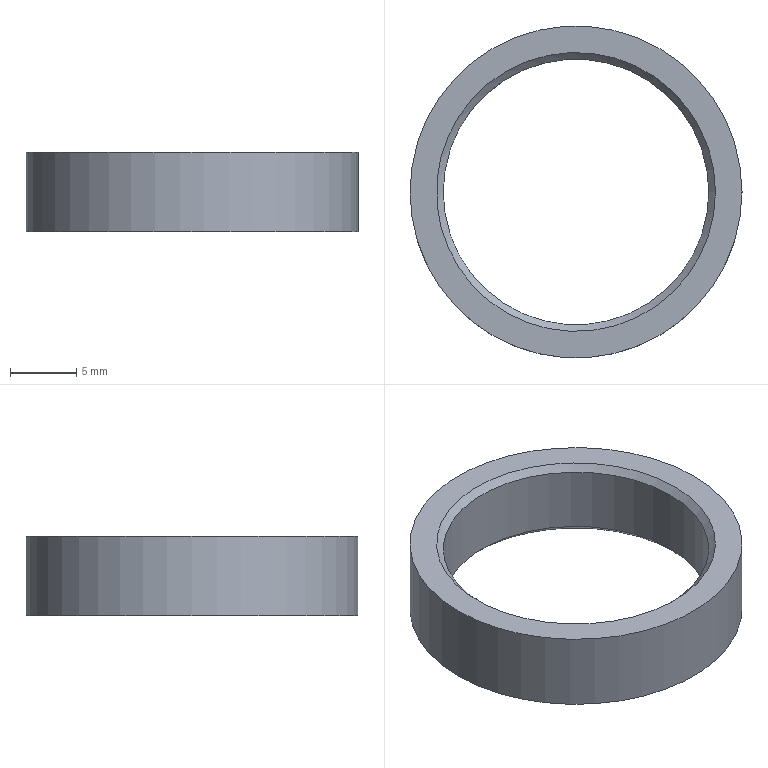Part | NX | features BREP 1 | 1 solid | 6 faces | box 25 x 25 x 6 mm | volume 1044 mm3 | cone 2 | cylinder 2 | plane 2 | commonest cylinder face diameters 20 x1 25 x1
STEP:
#1=CARTESIAN_POINT('',(10.5,0.,0.));
#2=VERTEX_POINT('',#1);
#3=CARTESIAN_POINT('',(0.,0.,0.));
#4=DIRECTION('',(0.,0.,1.));
#5=DIRECTION('',(1.,0.,0.));
#6=AXIS2_PLACEMENT_3D('',#3,#4,#5);
#7=CIRCLE('',#6,10.5);
#8=EDGE_CURVE('',#2,#2,#7,.T.);
#9=ORIENTED_EDGE('',*,*,#8,.F.);
#10=EDGE_LOOP('',(#9));
#11=FACE_BOUND('',#10,.T.);
#12=CARTESIAN_POINT('',(10.,0.,0.5));
#13=VERTEX_POINT('',#12);
#14=CARTESIAN_POINT('',(0.,0.,0.5));
#15=DIRECTION('',(0.,0.,-1.));
#16=DIRECTION('',(1.,0.,0.));
#17=AXIS2_PLACEMENT_3D('',#14,#15,#16);
#18=CIRCLE('',#17,10.);
#19=EDGE_CURVE('',#13,#13,#18,.T.);
#20=ORIENTED_EDGE('',*,*,#19,.F.);
#21=EDGE_LOOP('',(#20));
#22=FACE_BOUND('',#21,.T.);
#23=CARTESIAN_POINT('',(0.,0.,0.));
#24=DIRECTION('',(0.,0.,-1.));
#25=DIRECTION('',(-1.,0.,0.));
#26=AXIS2_PLACEMENT_3D('',#23,#24,#25);
#27=CONICAL_SURFACE('',#26,10.5,0.7854);
#28=ADVANCED_FACE('',(#11,#22),#27,.F.);
#29=CARTESIAN_POINT('',(10.5,0.,6.));
#30=VERTEX_POINT('',#29);
#31=CARTESIAN_POINT('',(0.,0.,6.));
#32=DIRECTION('',(0.,0.,-1.));
#33=DIRECTION('',(1.,0.,0.));
#34=AXIS2_PLACEMENT_3D('',#31,#32,#33);
#35=CIRCLE('',#34,10.5);
#36=EDGE_CURVE('',#30,#30,#35,.T.);
#37=ORIENTED_EDGE('',*,*,#36,.F.);
#38=EDGE_LOOP('',(#37));
#39=FACE_BOUND('',#38,.T.);
#40=CARTESIAN_POINT('',(10.,0.,5.5));
#41=VERTEX_POINT('',#40);
#42=CARTESIAN_POINT('',(0.,0.,5.5));
#43=DIRECTION('',(0.,0.,1.));
#44=DIRECTION('',(1.,0.,0.));
#45=AXIS2_PLACEMENT_3D('',#42,#43,#44);
#46=CIRCLE('',#45,10.);
#47=EDGE_CURVE('',#41,#41,#46,.T.);
#48=ORIENTED_EDGE('',*,*,#47,.F.);
#49=EDGE_LOOP('',(#48));
#50=FACE_BOUND('',#49,.T.);
#51=CARTESIAN_POINT('',(0.,0.,5.5));
#52=DIRECTION('',(0.,0.,1.));
#53=DIRECTION('',(1.,0.,0.));
#54=AXIS2_PLACEMENT_3D('',#51,#52,#53);
#55=CONICAL_SURFACE('',#54,10.,0.7854);
#56=ADVANCED_FACE('',(#39,#50),#55,.F.);
#57=ORIENTED_EDGE('',*,*,#19,.T.);
#58=EDGE_LOOP('',(#57));
#59=FACE_BOUND('',#58,.T.);
#60=ORIENTED_EDGE('',*,*,#47,.T.);
#61=EDGE_LOOP('',(#60));
#62=FACE_BOUND('',#61,.T.);
#63=CARTESIAN_POINT('',(0.,0.,6.));
#64=DIRECTION('',(0.,0.,-1.));
#65=DIRECTION('',(-1.,0.,0.));
#66=AXIS2_PLACEMENT_3D('',#63,#64,#65);
#67=CYLINDRICAL_SURFACE('',#66,10.);
#68=ADVANCED_FACE('',(#59,#62),#67,.F.);
#69=CARTESIAN_POINT('',(12.5,0.,0.));
#70=VERTEX_POINT('',#69);
#71=CARTESIAN_POINT('',(0.,0.,0.));
#72=DIRECTION('',(0.,0.,1.));
#73=DIRECTION('',(1.,0.,0.));
#74=AXIS2_PLACEMENT_3D('',#71,#72,#73);
#75=CIRCLE('',#74,12.5);
#76=EDGE_CURVE('',#70,#70,#75,.T.);
#77=ORIENTED_EDGE('',*,*,#76,.T.);
#78=EDGE_LOOP('',(#77));
#79=FACE_BOUND('',#78,.T.);
#80=CARTESIAN_POINT('',(12.5,0.,6.));
#81=VERTEX_POINT('',#80);
#82=CARTESIAN_POINT('',(0.,0.,6.));
#83=DIRECTION('',(0.,0.,1.));
#84=DIRECTION('',(1.,0.,0.));
#85=AXIS2_PLACEMENT_3D('',#82,#83,#84);
#86=CIRCLE('',#85,12.5);
#87=EDGE_CURVE('',#81,#81,#86,.T.);
#88=ORIENTED_EDGE('',*,*,#87,.F.);
#89=EDGE_LOOP('',(#88));
#90=FACE_BOUND('',#89,.T.);
#91=CARTESIAN_POINT('',(0.,0.,6.));
#92=DIRECTION('',(0.,0.,-1.));
#93=DIRECTION('',(-1.,0.,0.));
#94=AXIS2_PLACEMENT_3D('',#91,#92,#93);
#95=CYLINDRICAL_SURFACE('',#94,12.5);
#96=ADVANCED_FACE('',(#79,#90),#95,.T.);
#97=ORIENTED_EDGE('',*,*,#36,.T.);
#98=EDGE_LOOP('',(#97));
#99=FACE_BOUND('',#98,.T.);
#100=ORIENTED_EDGE('',*,*,#87,.T.);
#101=EDGE_LOOP('',(#100));
#102=FACE_BOUND('',#101,.T.);
#103=CARTESIAN_POINT('',(0.,0.,6.));
#104=DIRECTION('',(0.,0.,1.));
#105=DIRECTION('',(1.,0.,0.));
#106=AXIS2_PLACEMENT_3D('',#103,#104,#105);
#107=PLANE('',#106);
#108=ADVANCED_FACE('',(#99,#102),#107,.T.);
#109=ORIENTED_EDGE('',*,*,#8,.T.);
#110=EDGE_LOOP('',(#109));
#111=FACE_BOUND('',#110,.T.);
#112=ORIENTED_EDGE('',*,*,#76,.F.);
#113=EDGE_LOOP('',(#112));
#114=FACE_BOUND('',#113,.T.);
#115=CARTESIAN_POINT('',(0.,0.,0.));
#116=DIRECTION('',(0.,0.,1.));
#117=DIRECTION('',(1.,0.,0.));
#118=AXIS2_PLACEMENT_3D('',#115,#116,#117);
#119=PLANE('',#118);
#120=ADVANCED_FACE('',(#111,#114),#119,.F.);
#121=CLOSED_SHELL('',(#28,#56,#68,#96,#108,#120));
#122=MANIFOLD_SOLID_BREP('',#121);
#123=(LENGTH_UNIT()NAMED_UNIT(*)SI_UNIT(.MILLI.,.METRE.));
#124=UNCERTAINTY_MEASURE_WITH_UNIT(LENGTH_MEASURE(0.00001),#123,'','');
#125=(NAMED_UNIT(*)PLANE_ANGLE_UNIT()SI_UNIT($,.RADIAN.));
#126=(NAMED_UNIT(*)SI_UNIT($,.STERADIAN.)SOLID_ANGLE_UNIT());
#127=(GEOMETRIC_REPRESENTATION_CONTEXT(3)GLOBAL_UNCERTAINTY_ASSIGNED_CONTEXT((#124))GLOBAL_UNIT_ASSIGNED_CONTEXT((#123,#125,#126))REPRESENTATION_CONTEXT('',''));
#128=ADVANCED_BREP_SHAPE_REPRESENTATION('',(#122),#127);